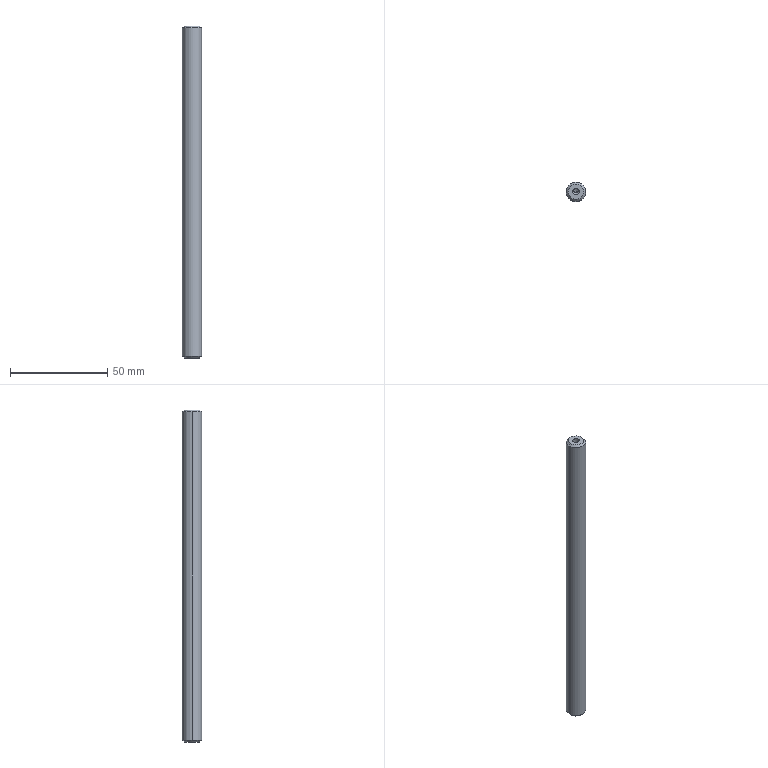Part | STEP file | PN_0005 Mount electronic clip support shaft | 1 solid | 16 faces | box 10 x 10 x 171 mm | volume 13199 mm3 | cone 8 | cylinder 6 | plane 2 | commonest cylinder face diameters 3.3 x4 10 x2
STEP:
#1=CARTESIAN_POINT('',(0.,0.,0.));
#2=DIRECTION('',(0.,0.,1.));
#3=DIRECTION('',(1.,0.,0.));
#4=AXIS2_PLACEMENT_3D('',#1,#2,#3);
#5=CARTESIAN_POINT('',(-1.65,0.,11.5));
#6=VERTEX_POINT('',#5);
#7=CARTESIAN_POINT('',(-1.65,0.,0.));
#8=VERTEX_POINT('',#7);
#9=CARTESIAN_POINT('',(-1.65,0.,0.));
#10=DIRECTION('',(0.,0.,-1.));
#11=VECTOR('',#10,1.);
#12=LINE('',#9,#11);
#13=CARTESIAN_POINT('',(0.,0.,0.));
#14=DIRECTION('',(0.,0.,-1.));
#15=DIRECTION('',(-1.,0.,0.));
#16=AXIS2_PLACEMENT_3D('',#13,#14,#15);
#17=CYLINDRICAL_SURFACE('',#16,1.65);
#18=CARTESIAN_POINT('',(6.283,0.));
#19=DIRECTION('',(0.,1.));
#20=VECTOR('',#19,1.);
#21=LINE('',#18,#20);
#22=(GEOMETRIC_REPRESENTATION_CONTEXT(2)PARAMETRIC_REPRESENTATION_CONTEXT()REPRESENTATION_CONTEXT('',''));
#23=DEFINITIONAL_REPRESENTATION('',(#21),#22);
#24=PCURVE('',#17,#23);
#25=CARTESIAN_POINT('',(0.,0.,0.));
#26=DIRECTION('',(0.,0.,-1.));
#27=DIRECTION('',(-1.,0.,0.));
#28=AXIS2_PLACEMENT_3D('',#25,#26,#27);
#29=CYLINDRICAL_SURFACE('',#28,1.65);
#30=CARTESIAN_POINT('',(0.,0.));
#31=DIRECTION('',(0.,1.));
#32=VECTOR('',#31,1.);
#33=LINE('',#30,#32);
#34=(GEOMETRIC_REPRESENTATION_CONTEXT(2)PARAMETRIC_REPRESENTATION_CONTEXT()REPRESENTATION_CONTEXT('',''));
#35=DEFINITIONAL_REPRESENTATION('',(#33),#34);
#36=PCURVE('',#29,#35);
#37=SURFACE_CURVE('',#12,(#24,#36),.PCURVE_S1.);
#38=EDGE_CURVE('',#6,#8,#37,.T.);
#39=ORIENTED_EDGE('',*,*,#38,.T.);
#40=CARTESIAN_POINT('',(1.65,0.,0.));
#41=VERTEX_POINT('',#40);
#42=CARTESIAN_POINT('',(0.,0.,0.));
#43=DIRECTION('',(0.,0.,-1.));
#44=DIRECTION('',(-1.,0.,0.));
#45=AXIS2_PLACEMENT_3D('',#42,#43,#44);
#46=CIRCLE('',#45,1.65);
#47=CARTESIAN_POINT('',(0.,0.));
#48=DIRECTION('',(1.,0.));
#49=VECTOR('',#48,1.);
#50=LINE('',#47,#49);
#51=(GEOMETRIC_REPRESENTATION_CONTEXT(2)PARAMETRIC_REPRESENTATION_CONTEXT()REPRESENTATION_CONTEXT('',''));
#52=DEFINITIONAL_REPRESENTATION('',(#50),#51);
#53=PCURVE('',#17,#52);
#54=CARTESIAN_POINT('',(0.,0.,0.));
#55=DIRECTION('',(0.,0.,1.));
#56=DIRECTION('',(1.,0.,0.));
#57=AXIS2_PLACEMENT_3D('',#54,#55,#56);
#58=PLANE('',#57);
#59=CARTESIAN_POINT('',(-1.65,0.));
#60=CARTESIAN_POINT('',(-1.65,2.858));
#61=CARTESIAN_POINT('',(0.825,1.429));
#62=CARTESIAN_POINT('',(3.3,0.));
#63=CARTESIAN_POINT('',(0.825,-1.429));
#64=CARTESIAN_POINT('',(-1.65,-2.858));
#65=CARTESIAN_POINT('',(-1.65,0.));
#66=(BOUNDED_CURVE()B_SPLINE_CURVE(2,(#59,#60,#61,#62,#63,#64,#65),.UNSPECIFIED.,.T.,.F.)B_SPLINE_CURVE_WITH_KNOTS((1,2,2,2,2,1),(-2.094,0.,2.094,4.189,6.283,8.378),.UNSPECIFIED.)CURVE()GEOMETRIC_REPRESENTATION_ITEM()RATIONAL_B_SPLINE_CURVE((1.,0.5,1.,0.5,1.,0.5,1.))REPRESENTATION_ITEM(''));
#67=(GEOMETRIC_REPRESENTATION_CONTEXT(2)PARAMETRIC_REPRESENTATION_CONTEXT()REPRESENTATION_CONTEXT('',''));
#68=DEFINITIONAL_REPRESENTATION('',(#66),#67);
#69=PCURVE('',#58,#68);
#70=SURFACE_CURVE('',#46,(#53,#69),.PCURVE_S1.);
#71=EDGE_CURVE('',#41,#8,#70,.T.);
#72=ORIENTED_EDGE('',*,*,#71,.F.);
#73=CARTESIAN_POINT('',(1.65,0.,11.5));
#74=VERTEX_POINT('',#73);
#75=CARTESIAN_POINT('',(1.65,0.,0.));
#76=DIRECTION('',(0.,0.,-1.));
#77=VECTOR('',#76,1.);
#78=LINE('',#75,#77);
#79=CARTESIAN_POINT('',(3.142,0.));
#80=DIRECTION('',(0.,1.));
#81=VECTOR('',#80,1.);
#82=LINE('',#79,#81);
#83=(GEOMETRIC_REPRESENTATION_CONTEXT(2)PARAMETRIC_REPRESENTATION_CONTEXT()REPRESENTATION_CONTEXT('',''));
#84=DEFINITIONAL_REPRESENTATION('',(#82),#83);
#85=PCURVE('',#17,#84);
#86=CARTESIAN_POINT('',(3.142,0.));
#87=DIRECTION('',(0.,1.));
#88=VECTOR('',#87,1.);
#89=LINE('',#86,#88);
#90=(GEOMETRIC_REPRESENTATION_CONTEXT(2)PARAMETRIC_REPRESENTATION_CONTEXT()REPRESENTATION_CONTEXT('',''));
#91=DEFINITIONAL_REPRESENTATION('',(#89),#90);
#92=PCURVE('',#29,#91);
#93=SURFACE_CURVE('',#78,(#85,#92),.PCURVE_S1.);
#94=EDGE_CURVE('',#74,#41,#93,.T.);
#95=ORIENTED_EDGE('',*,*,#94,.F.);
#96=CARTESIAN_POINT('',(0.,0.,11.5));
#97=DIRECTION('',(0.,0.,-1.));
#98=DIRECTION('',(-1.,0.,0.));
#99=AXIS2_PLACEMENT_3D('',#96,#97,#98);
#100=CIRCLE('',#99,1.65);
#101=CARTESIAN_POINT('',(0.,-11.5));
#102=DIRECTION('',(1.,0.));
#103=VECTOR('',#102,1.);
#104=LINE('',#101,#103);
#105=(GEOMETRIC_REPRESENTATION_CONTEXT(2)PARAMETRIC_REPRESENTATION_CONTEXT()REPRESENTATION_CONTEXT('',''));
#106=DEFINITIONAL_REPRESENTATION('',(#104),#105);
#107=PCURVE('',#17,#106);
#108=CARTESIAN_POINT('',(0.,0.,11.5));
#109=DIRECTION('',(0.,0.,-1.));
#110=DIRECTION('',(-1.,0.,0.));
#111=AXIS2_PLACEMENT_3D('',#108,#109,#110);
#112=CONICAL_SURFACE('',#111,1.65,1.03);
#113=CARTESIAN_POINT('',(0.,0.));
#114=DIRECTION('',(1.,0.));
#115=VECTOR('',#114,1.);
#116=LINE('',#113,#115);
#117=(GEOMETRIC_REPRESENTATION_CONTEXT(2)PARAMETRIC_REPRESENTATION_CONTEXT()REPRESENTATION_CONTEXT('',''));
#118=DEFINITIONAL_REPRESENTATION('',(#116),#117);
#119=PCURVE('',#112,#118);
#120=SURFACE_CURVE('',#100,(#107,#119),.PCURVE_S1.);
#121=EDGE_CURVE('',#74,#6,#120,.T.);
#122=ORIENTED_EDGE('',*,*,#121,.T.);
#123=EDGE_LOOP('',(#39,#72,#95,#122));
#124=FACE_BOUND('',#123,.F.);
#125=ADVANCED_FACE('',(#124),#17,.F.);
#126=ORIENTED_EDGE('',*,*,#121,.F.);
#127=CARTESIAN_POINT('',(0.,0.,12.491));
#128=VERTEX_POINT('',#127);
#129=CARTESIAN_POINT('',(1.65,0.,11.5));
#130=DIRECTION('',(0.8572,0.,-0.515));
#131=VECTOR('',#130,1.);
#132=LINE('',#129,#131);
#133=CARTESIAN_POINT('',(3.142,0.));
#134=DIRECTION('',(0.,1.));
#135=VECTOR('',#134,1.);
#136=LINE('',#133,#135);
#137=(GEOMETRIC_REPRESENTATION_CONTEXT(2)PARAMETRIC_REPRESENTATION_CONTEXT()REPRESENTATION_CONTEXT('',''));
#138=DEFINITIONAL_REPRESENTATION('',(#136),#137);
#139=PCURVE('',#112,#138);
#140=CARTESIAN_POINT('',(0.,0.,11.5));
#141=DIRECTION('',(0.,0.,-1.));
#142=DIRECTION('',(-1.,0.,0.));
#143=AXIS2_PLACEMENT_3D('',#140,#141,#142);
#144=CONICAL_SURFACE('',#143,1.65,1.03);
#145=CARTESIAN_POINT('',(3.142,0.));
#146=DIRECTION('',(0.,1.));
#147=VECTOR('',#146,1.);
#148=LINE('',#145,#147);
#149=(GEOMETRIC_REPRESENTATION_CONTEXT(2)PARAMETRIC_REPRESENTATION_CONTEXT()REPRESENTATION_CONTEXT('',''));
#150=DEFINITIONAL_REPRESENTATION('',(#148),#149);
#151=PCURVE('',#144,#150);
#152=SURFACE_CURVE('',#132,(#139,#151),.PCURVE_S1.);
#153=EDGE_CURVE('',#128,#74,#152,.T.);
#154=ORIENTED_EDGE('',*,*,#153,.F.);
#155=CARTESIAN_POINT('',(-1.65,0.,11.5));
#156=DIRECTION('',(-0.8572,0.,-0.515));
#157=VECTOR('',#156,1.);
#158=LINE('',#155,#157);
#159=CARTESIAN_POINT('',(6.283,0.));
#160=DIRECTION('',(0.,1.));
#161=VECTOR('',#160,1.);
#162=LINE('',#159,#161);
#163=(GEOMETRIC_REPRESENTATION_CONTEXT(2)PARAMETRIC_REPRESENTATION_CONTEXT()REPRESENTATION_CONTEXT('',''));
#164=DEFINITIONAL_REPRESENTATION('',(#162),#163);
#165=PCURVE('',#112,#164);
#166=CARTESIAN_POINT('',(0.,0.));
#167=DIRECTION('',(0.,1.));
#168=VECTOR('',#167,1.);
#169=LINE('',#166,#168);
#170=(GEOMETRIC_REPRESENTATION_CONTEXT(2)PARAMETRIC_REPRESENTATION_CONTEXT()REPRESENTATION_CONTEXT('',''));
#171=DEFINITIONAL_REPRESENTATION('',(#169),#170);
#172=PCURVE('',#144,#171);
#173=SURFACE_CURVE('',#158,(#165,#172),.PCURVE_S1.);
#174=EDGE_CURVE('',#128,#6,#173,.T.);
#175=ORIENTED_EDGE('',*,*,#174,.T.);
#176=EDGE_LOOP('',(#126,#154,#175));
#177=FACE_BOUND('',#176,.F.);
#178=ADVANCED_FACE('',(#177),#112,.F.);
#179=CARTESIAN_POINT('',(1.65,0.,159.5));
#180=VERTEX_POINT('',#179);
#181=CARTESIAN_POINT('',(1.65,0.,171.));
#182=VERTEX_POINT('',#181);
#183=CARTESIAN_POINT('',(1.65,0.,171.));
#184=DIRECTION('',(0.,0.,1.));
#185=VECTOR('',#184,1.);
#186=LINE('',#183,#185);
#187=CARTESIAN_POINT('',(0.,0.,171.));
#188=DIRECTION('',(0.,0.,1.));
#189=DIRECTION('',(1.,0.,0.));
#190=AXIS2_PLACEMENT_3D('',#187,#188,#189);
#191=CYLINDRICAL_SURFACE('',#190,1.65);
#192=CARTESIAN_POINT('',(6.283,0.));
#193=DIRECTION('',(0.,1.));
#194=VECTOR('',#193,1.);
#195=LINE('',#192,#194);
#196=(GEOMETRIC_REPRESENTATION_CONTEXT(2)PARAMETRIC_REPRESENTATION_CONTEXT()REPRESENTATION_CONTEXT('',''));
#197=DEFINITIONAL_REPRESENTATION('',(#195),#196);
#198=PCURVE('',#191,#197);
#199=CARTESIAN_POINT('',(0.,0.,171.));
#200=DIRECTION('',(0.,0.,1.));
#201=DIRECTION('',(1.,0.,0.));
#202=AXIS2_PLACEMENT_3D('',#199,#200,#201);
#203=CYLINDRICAL_SURFACE('',#202,1.65);
#204=CARTESIAN_POINT('',(0.,0.));
#205=DIRECTION('',(0.,1.));
#206=VECTOR('',#205,1.);
#207=LINE('',#204,#206);
#208=(GEOMETRIC_REPRESENTATION_CONTEXT(2)PARAMETRIC_REPRESENTATION_CONTEXT()REPRESENTATION_CONTEXT('',''));
#209=DEFINITIONAL_REPRESENTATION('',(#207),#208);
#210=PCURVE('',#203,#209);
#211=SURFACE_CURVE('',#186,(#198,#210),.PCURVE_S1.);
#212=EDGE_CURVE('',#180,#182,#211,.T.);
#213=ORIENTED_EDGE('',*,*,#212,.T.);
#214=CARTESIAN_POINT('',(-1.65,0.,171.));
#215=VERTEX_POINT('',#214);
#216=CARTESIAN_POINT('',(0.,0.,171.));
#217=DIRECTION('',(0.,0.,1.));
#218=DIRECTION('',(1.,0.,0.));
#219=AXIS2_PLACEMENT_3D('',#216,#217,#218);
#220=CIRCLE('',#219,1.65);
#221=CARTESIAN_POINT('',(0.,0.));
#222=DIRECTION('',(1.,0.));
#223=VECTOR('',#222,1.);
#224=LINE('',#221,#223);
#225=(GEOMETRIC_REPRESENTATION_CONTEXT(2)PARAMETRIC_REPRESENTATION_CONTEXT()REPRESENTATION_CONTEXT('',''));
#226=DEFINITIONAL_REPRESENTATION('',(#224),#225);
#227=PCURVE('',#191,#226);
#228=CARTESIAN_POINT('',(0.,0.,171.));
#229=DIRECTION('',(0.,0.,1.));
#230=DIRECTION('',(1.,0.,0.));
#231=AXIS2_PLACEMENT_3D('',#228,#229,#230);
#232=PLANE('',#231);
#233=CARTESIAN_POINT('',(0.,0.));
#234=DIRECTION('',(1.,0.));
#235=AXIS2_PLACEMENT_2D('',#233,#234);
#236=CIRCLE('',#235,1.65);
#237=(GEOMETRIC_REPRESENTATION_CONTEXT(2)PARAMETRIC_REPRESENTATION_CONTEXT()REPRESENTATION_CONTEXT('',''));
#238=DEFINITIONAL_REPRESENTATION('',(#236),#237);
#239=PCURVE('',#232,#238);
#240=SURFACE_CURVE('',#220,(#227,#239),.PCURVE_S1.);
#241=EDGE_CURVE('',#215,#182,#240,.T.);
#242=ORIENTED_EDGE('',*,*,#241,.F.);
#243=CARTESIAN_POINT('',(-1.65,0.,159.5));
#244=VERTEX_POINT('',#243);
#245=CARTESIAN_POINT('',(-1.65,0.,171.));
#246=DIRECTION('',(0.,0.,1.));
#247=VECTOR('',#246,1.);
#248=LINE('',#245,#247);
#249=CARTESIAN_POINT('',(3.142,0.));
#250=DIRECTION('',(0.,1.));
#251=VECTOR('',#250,1.);
#252=LINE('',#249,#251);
#253=(GEOMETRIC_REPRESENTATION_CONTEXT(2)PARAMETRIC_REPRESENTATION_CONTEXT()REPRESENTATION_CONTEXT('',''));
#254=DEFINITIONAL_REPRESENTATION('',(#252),#253);
#255=PCURVE('',#191,#254);
#256=CARTESIAN_POINT('',(3.142,0.));
#257=DIRECTION('',(0.,1.));
#258=VECTOR('',#257,1.);
#259=LINE('',#256,#258);
#260=(GEOMETRIC_REPRESENTATION_CONTEXT(2)PARAMETRIC_REPRESENTATION_CONTEXT()REPRESENTATION_CONTEXT('',''));
#261=DEFINITIONAL_REPRESENTATION('',(#259),#260);
#262=PCURVE('',#203,#261);
#263=SURFACE_CURVE('',#248,(#255,#262),.PCURVE_S1.);
#264=EDGE_CURVE('',#244,#215,#263,.T.);
#265=ORIENTED_EDGE('',*,*,#264,.F.);
#266=CARTESIAN_POINT('',(0.,0.,159.5));
#267=DIRECTION('',(0.,0.,1.));
#268=DIRECTION('',(1.,0.,0.));
#269=AXIS2_PLACEMENT_3D('',#266,#267,#268);
#270=CIRCLE('',#269,1.65);
#271=CARTESIAN_POINT('',(0.,-11.5));
#272=DIRECTION('',(1.,0.));
#273=VECTOR('',#272,1.);
#274=LINE('',#271,#273);
#275=(GEOMETRIC_REPRESENTATION_CONTEXT(2)PARAMETRIC_REPRESENTATION_CONTEXT()REPRESENTATION_CONTEXT('',''));
#276=DEFINITIONAL_REPRESENTATION('',(#274),#275);
#277=PCURVE('',#191,#276);
#278=CARTESIAN_POINT('',(0.,0.,159.5));
#279=DIRECTION('',(0.,0.,1.));
#280=DIRECTION('',(1.,0.,0.));
#281=AXIS2_PLACEMENT_3D('',#278,#279,#280);
#282=CONICAL_SURFACE('',#281,1.65,1.03);
#283=CARTESIAN_POINT('',(0.,0.));
#284=DIRECTION('',(1.,0.));
#285=VECTOR('',#284,1.);
#286=LINE('',#283,#285);
#287=(GEOMETRIC_REPRESENTATION_CONTEXT(2)PARAMETRIC_REPRESENTATION_CONTEXT()REPRESENTATION_CONTEXT('',''));
#288=DEFINITIONAL_REPRESENTATION('',(#286),#287);
#289=PCURVE('',#282,#288);
#290=SURFACE_CURVE('',#270,(#277,#289),.PCURVE_S1.);
#291=EDGE_CURVE('',#244,#180,#290,.T.);
#292=ORIENTED_EDGE('',*,*,#291,.T.);
#293=EDGE_LOOP('',(#213,#242,#265,#292));
#294=FACE_BOUND('',#293,.F.);
#295=ADVANCED_FACE('',(#294),#191,.F.);
#296=ORIENTED_EDGE('',*,*,#291,.F.);
#297=CARTESIAN_POINT('',(0.,0.,158.509));
#298=VERTEX_POINT('',#297);
#299=CARTESIAN_POINT('',(-1.65,0.,159.5));
#300=DIRECTION('',(-0.8572,0.,0.515));
#301=VECTOR('',#300,1.);
#302=LINE('',#299,#301);
#303=CARTESIAN_POINT('',(3.142,0.));
#304=DIRECTION('',(0.,1.));
#305=VECTOR('',#304,1.);
#306=LINE('',#303,#305);
#307=(GEOMETRIC_REPRESENTATION_CONTEXT(2)PARAMETRIC_REPRESENTATION_CONTEXT()REPRESENTATION_CONTEXT('',''));
#308=DEFINITIONAL_REPRESENTATION('',(#306),#307);
#309=PCURVE('',#282,#308);
#310=CARTESIAN_POINT('',(0.,0.,159.5));
#311=DIRECTION('',(0.,0.,1.));
#312=DIRECTION('',(1.,0.,0.));
#313=AXIS2_PLACEMENT_3D('',#310,#311,#312);
#314=CONICAL_SURFACE('',#313,1.65,1.03);
#315=CARTESIAN_POINT('',(3.142,0.));
#316=DIRECTION('',(0.,1.));
#317=VECTOR('',#316,1.);
#318=LINE('',#315,#317);
#319=(GEOMETRIC_REPRESENTATION_CONTEXT(2)PARAMETRIC_REPRESENTATION_CONTEXT()REPRESENTATION_CONTEXT('',''));
#320=DEFINITIONAL_REPRESENTATION('',(#318),#319);
#321=PCURVE('',#314,#320);
#322=SURFACE_CURVE('',#302,(#309,#321),.PCURVE_S1.);
#323=EDGE_CURVE('',#298,#244,#322,.T.);
#324=ORIENTED_EDGE('',*,*,#323,.F.);
#325=CARTESIAN_POINT('',(1.65,0.,159.5));
#326=DIRECTION('',(0.8572,0.,0.515));
#327=VECTOR('',#326,1.);
#328=LINE('',#325,#327);
#329=CARTESIAN_POINT('',(6.283,0.));
#330=DIRECTION('',(0.,1.));
#331=VECTOR('',#330,1.);
#332=LINE('',#329,#331);
#333=(GEOMETRIC_REPRESENTATION_CONTEXT(2)PARAMETRIC_REPRESENTATION_CONTEXT()REPRESENTATION_CONTEXT('',''));
#334=DEFINITIONAL_REPRESENTATION('',(#332),#333);
#335=PCURVE('',#282,#334);
#336=CARTESIAN_POINT('',(0.,0.));
#337=DIRECTION('',(0.,1.));
#338=VECTOR('',#337,1.);
#339=LINE('',#336,#338);
#340=(GEOMETRIC_REPRESENTATION_CONTEXT(2)PARAMETRIC_REPRESENTATION_CONTEXT()REPRESENTATION_CONTEXT('',''));
#341=DEFINITIONAL_REPRESENTATION('',(#339),#340);
#342=PCURVE('',#314,#341);
#343=SURFACE_CURVE('',#328,(#335,#342),.PCURVE_S1.);
#344=EDGE_CURVE('',#298,#180,#343,.T.);
#345=ORIENTED_EDGE('',*,*,#344,.T.);
#346=EDGE_LOOP('',(#296,#324,#345));
#347=FACE_BOUND('',#346,.F.);
#348=ADVANCED_FACE('',(#347),#282,.F.);
#349=CARTESIAN_POINT('',(4.,0.,171.));
#350=VERTEX_POINT('',#349);
#351=CARTESIAN_POINT('',(-4.,0.,171.));
#352=VERTEX_POINT('',#351);
#353=CARTESIAN_POINT('',(0.,0.,171.));
#354=DIRECTION('',(0.,0.,1.));
#355=DIRECTION('',(1.,0.,0.));
#356=AXIS2_PLACEMENT_3D('',#353,#354,#355);
#357=CIRCLE('',#356,4.);
#358=CARTESIAN_POINT('',(0.,0.,171.));
#359=DIRECTION('',(0.,0.,-1.));
#360=DIRECTION('',(-1.,0.,0.));
#361=AXIS2_PLACEMENT_3D('',#358,#359,#360);
#362=CONICAL_SURFACE('',#361,4.,0.7854);
#363=CARTESIAN_POINT('',(3.142,0.));
#364=DIRECTION('',(-1.,0.));
#365=VECTOR('',#364,1.);
#366=LINE('',#363,#365);
#367=(GEOMETRIC_REPRESENTATION_CONTEXT(2)PARAMETRIC_REPRESENTATION_CONTEXT()REPRESENTATION_CONTEXT('',''));
#368=DEFINITIONAL_REPRESENTATION('',(#366),#367);
#369=PCURVE('',#362,#368);
#370=CARTESIAN_POINT('',(0.,0.));
#371=DIRECTION('',(1.,0.));
#372=AXIS2_PLACEMENT_2D('',#370,#371);
#373=CIRCLE('',#372,4.);
#374=(GEOMETRIC_REPRESENTATION_CONTEXT(2)PARAMETRIC_REPRESENTATION_CONTEXT()REPRESENTATION_CONTEXT('',''));
#375=DEFINITIONAL_REPRESENTATION('',(#373),#374);
#376=PCURVE('',#232,#375);
#377=SURFACE_CURVE('',#357,(#369,#376),.PCURVE_S1.);
#378=EDGE_CURVE('',#350,#352,#377,.T.);
#379=ORIENTED_EDGE('',*,*,#378,.F.);
#380=CARTESIAN_POINT('',(5.,0.,170.));
#381=VERTEX_POINT('',#380);
#382=CARTESIAN_POINT('',(4.,0.,171.));
#383=DIRECTION('',(0.7071,0.,-0.7071));
#384=VECTOR('',#383,1.);
#385=LINE('',#382,#384);
#386=CARTESIAN_POINT('',(3.142,0.));
#387=DIRECTION('',(0.,1.));
#388=VECTOR('',#387,1.);
#389=LINE('',#386,#388);
#390=(GEOMETRIC_REPRESENTATION_CONTEXT(2)PARAMETRIC_REPRESENTATION_CONTEXT()REPRESENTATION_CONTEXT('',''));
#391=DEFINITIONAL_REPRESENTATION('',(#389),#390);
#392=PCURVE('',#362,#391);
#393=CARTESIAN_POINT('',(0.,0.,171.));
#394=DIRECTION('',(0.,0.,-1.));
#395=DIRECTION('',(-1.,0.,0.));
#396=AXIS2_PLACEMENT_3D('',#393,#394,#395);
#397=CONICAL_SURFACE('',#396,4.,0.7854);
#398=CARTESIAN_POINT('',(3.142,0.));
#399=DIRECTION('',(0.,1.));
#400=VECTOR('',#399,1.);
#401=LINE('',#398,#400);
#402=(GEOMETRIC_REPRESENTATION_CONTEXT(2)PARAMETRIC_REPRESENTATION_CONTEXT()REPRESENTATION_CONTEXT('',''));
#403=DEFINITIONAL_REPRESENTATION('',(#401),#402);
#404=PCURVE('',#397,#403);
#405=SURFACE_CURVE('',#385,(#392,#404),.PCURVE_S1.);
#406=EDGE_CURVE('',#350,#381,#405,.T.);
#407=ORIENTED_EDGE('',*,*,#406,.T.);
#408=CARTESIAN_POINT('',(-5.,0.,170.));
#409=VERTEX_POINT('',#408);
#410=CARTESIAN_POINT('',(0.,0.,170.));
#411=DIRECTION('',(0.,0.,-1.));
#412=DIRECTION('',(1.,0.,0.));
#413=AXIS2_PLACEMENT_3D('',#410,#411,#412);
#414=CIRCLE('',#413,5.);
#415=CARTESIAN_POINT('',(-3.142,1.));
#416=DIRECTION('',(1.,0.));
#417=VECTOR('',#416,1.);
#418=LINE('',#415,#417);
#419=(GEOMETRIC_REPRESENTATION_CONTEXT(2)PARAMETRIC_REPRESENTATION_CONTEXT()REPRESENTATION_CONTEXT('',''));
#420=DEFINITIONAL_REPRESENTATION('',(#418),#419);
#421=PCURVE('',#362,#420);
#422=CARTESIAN_POINT('',(0.,0.,171.));
#423=DIRECTION('',(0.,0.,-1.));
#424=DIRECTION('',(-1.,0.,0.));
#425=AXIS2_PLACEMENT_3D('',#422,#423,#424);
#426=CYLINDRICAL_SURFACE('',#425,5.);
#427=CARTESIAN_POINT('',(-3.142,1.));
#428=DIRECTION('',(1.,0.));
#429=VECTOR('',#428,1.);
#430=LINE('',#427,#429);
#431=(GEOMETRIC_REPRESENTATION_CONTEXT(2)PARAMETRIC_REPRESENTATION_CONTEXT()REPRESENTATION_CONTEXT('',''));
#432=DEFINITIONAL_REPRESENTATION('',(#430),#431);
#433=PCURVE('',#426,#432);
#434=SURFACE_CURVE('',#414,(#421,#433),.PCURVE_S1.);
#435=EDGE_CURVE('',#409,#381,#434,.T.);
#436=ORIENTED_EDGE('',*,*,#435,.F.);
#437=CARTESIAN_POINT('',(-4.,0.,171.));
#438=DIRECTION('',(-0.7071,0.,-0.7071));
#439=VECTOR('',#438,1.);
#440=LINE('',#437,#439);
#441=CARTESIAN_POINT('',(0.,0.));
#442=DIRECTION('',(0.,1.));
#443=VECTOR('',#442,1.);
#444=LINE('',#441,#443);
#445=(GEOMETRIC_REPRESENTATION_CONTEXT(2)PARAMETRIC_REPRESENTATION_CONTEXT()REPRESENTATION_CONTEXT('',''));
#446=DEFINITIONAL_REPRESENTATION('',(#444),#445);
#447=PCURVE('',#362,#446);
#448=CARTESIAN_POINT('',(6.283,0.));
#449=DIRECTION('',(0.,1.));
#450=VECTOR('',#449,1.);
#451=LINE('',#448,#450);
#452=(GEOMETRIC_REPRESENTATION_CONTEXT(2)PARAMETRIC_REPRESENTATION_CONTEXT()REPRESENTATION_CONTEXT('',''));
#453=DEFINITIONAL_REPRESENTATION('',(#451),#452);
#454=PCURVE('',#397,#453);
#455=SURFACE_CURVE('',#440,(#447,#454),.PCURVE_S1.);
#456=EDGE_CURVE('',#352,#409,#455,.T.);
#457=ORIENTED_EDGE('',*,*,#456,.F.);
#458=EDGE_LOOP('',(#379,#407,#436,#457));
#459=FACE_BOUND('',#458,.T.);
#460=ADVANCED_FACE('',(#459),#362,.T.);
#461=CARTESIAN_POINT('',(-4.,0.,0.));
#462=VERTEX_POINT('',#461);
#463=CARTESIAN_POINT('',(4.,0.,0.));
#464=VERTEX_POINT('',#463);
#465=CARTESIAN_POINT('',(0.,0.,0.));
#466=DIRECTION('',(0.,0.,-1.));
#467=DIRECTION('',(1.,0.,0.));
#468=AXIS2_PLACEMENT_3D('',#465,#466,#467);
#469=CIRCLE('',#468,4.);
#470=CARTESIAN_POINT('',(0.,0.,1.));
#471=DIRECTION('',(0.,0.,1.));
#472=DIRECTION('',(1.,0.,0.));
#473=AXIS2_PLACEMENT_3D('',#470,#471,#472);
#474=CONICAL_SURFACE('',#473,5.,0.7854);
#475=CARTESIAN_POINT('',(6.283,-1.));
#476=DIRECTION('',(-1.,0.));
#477=VECTOR('',#476,1.);
#478=LINE('',#475,#477);
#479=(GEOMETRIC_REPRESENTATION_CONTEXT(2)PARAMETRIC_REPRESENTATION_CONTEXT()REPRESENTATION_CONTEXT('',''));
#480=DEFINITIONAL_REPRESENTATION('',(#478),#479);
#481=PCURVE('',#474,#480);
#482=CARTESIAN_POINT('',(4.,0.));
#483=CARTESIAN_POINT('',(4.,-6.928));
#484=CARTESIAN_POINT('',(-2.,-3.464));
#485=CARTESIAN_POINT('',(-8.,0.));
#486=CARTESIAN_POINT('',(-2.,3.464));
#487=CARTESIAN_POINT('',(4.,6.928));
#488=CARTESIAN_POINT('',(4.,0.));
#489=(BOUNDED_CURVE()B_SPLINE_CURVE(2,(#482,#483,#484,#485,#486,#487,#488),.UNSPECIFIED.,.T.,.F.)B_SPLINE_CURVE_WITH_KNOTS((1,2,2,2,2,1),(-2.094,0.,2.094,4.189,6.283,8.378),.UNSPECIFIED.)CURVE()GEOMETRIC_REPRESENTATION_ITEM()RATIONAL_B_SPLINE_CURVE((1.,0.5,1.,0.5,1.,0.5,1.))REPRESENTATION_ITEM(''));
#490=(GEOMETRIC_REPRESENTATION_CONTEXT(2)PARAMETRIC_REPRESENTATION_CONTEXT()REPRESENTATION_CONTEXT('',''));
#491=DEFINITIONAL_REPRESENTATION('',(#489),#490);
#492=PCURVE('',#58,#491);
#493=SURFACE_CURVE('',#469,(#481,#492),.PCURVE_S1.);
#494=EDGE_CURVE('',#462,#464,#493,.T.);
#495=ORIENTED_EDGE('',*,*,#494,.F.);
#496=CARTESIAN_POINT('',(-5.,0.,1.));
#497=VERTEX_POINT('',#496);
#498=CARTESIAN_POINT('',(-5.,0.,1.));
#499=DIRECTION('',(-0.7071,0.,0.7071));
#500=VECTOR('',#499,1.);
#501=LINE('',#498,#500);
#502=CARTESIAN_POINT('',(3.142,0.));
#503=DIRECTION('',(0.,1.));
#504=VECTOR('',#503,1.);
#505=LINE('',#502,#504);
#506=(GEOMETRIC_REPRESENTATION_CONTEXT(2)PARAMETRIC_REPRESENTATION_CONTEXT()REPRESENTATION_CONTEXT('',''));
#507=DEFINITIONAL_REPRESENTATION('',(#505),#506);
#508=PCURVE('',#474,#507);
#509=CARTESIAN_POINT('',(0.,0.,1.));
#510=DIRECTION('',(0.,0.,1.));
#511=DIRECTION('',(1.,0.,0.));
#512=AXIS2_PLACEMENT_3D('',#509,#510,#511);
#513=CONICAL_SURFACE('',#512,5.,0.7854);
#514=CARTESIAN_POINT('',(3.142,0.));
#515=DIRECTION('',(0.,1.));
#516=VECTOR('',#515,1.);
#517=LINE('',#514,#516);
#518=(GEOMETRIC_REPRESENTATION_CONTEXT(2)PARAMETRIC_REPRESENTATION_CONTEXT()REPRESENTATION_CONTEXT('',''));
#519=DEFINITIONAL_REPRESENTATION('',(#517),#518);
#520=PCURVE('',#513,#519);
#521=SURFACE_CURVE('',#501,(#508,#520),.PCURVE_S1.);
#522=EDGE_CURVE('',#462,#497,#521,.T.);
#523=ORIENTED_EDGE('',*,*,#522,.T.);
#524=CARTESIAN_POINT('',(5.,0.,1.));
#525=VERTEX_POINT('',#524);
#526=CARTESIAN_POINT('',(0.,0.,1.));
#527=DIRECTION('',(0.,0.,1.));
#528=DIRECTION('',(1.,0.,0.));
#529=AXIS2_PLACEMENT_3D('',#526,#527,#528);
#530=CIRCLE('',#529,5.);
#531=CARTESIAN_POINT('',(0.,0.));
#532=DIRECTION('',(1.,0.));
#533=VECTOR('',#532,1.);
#534=LINE('',#531,#533);
#535=(GEOMETRIC_REPRESENTATION_CONTEXT(2)PARAMETRIC_REPRESENTATION_CONTEXT()REPRESENTATION_CONTEXT('',''));
#536=DEFINITIONAL_REPRESENTATION('',(#534),#535);
#537=PCURVE('',#474,#536);
#538=CARTESIAN_POINT('',(3.142,170.));
#539=DIRECTION('',(-1.,0.));
#540=VECTOR('',#539,1.);
#541=LINE('',#538,#540);
#542=(GEOMETRIC_REPRESENTATION_CONTEXT(2)PARAMETRIC_REPRESENTATION_CONTEXT()REPRESENTATION_CONTEXT('',''));
#543=DEFINITIONAL_REPRESENTATION('',(#541),#542);
#544=PCURVE('',#426,#543);
#545=SURFACE_CURVE('',#530,(#537,#544),.PCURVE_S1.);
#546=EDGE_CURVE('',#525,#497,#545,.T.);
#547=ORIENTED_EDGE('',*,*,#546,.F.);
#548=CARTESIAN_POINT('',(5.,0.,1.));
#549=DIRECTION('',(0.7071,0.,0.7071));
#550=VECTOR('',#549,1.);
#551=LINE('',#548,#550);
#552=CARTESIAN_POINT('',(0.,0.));
#553=DIRECTION('',(0.,1.));
#554=VECTOR('',#553,1.);
#555=LINE('',#552,#554);
#556=(GEOMETRIC_REPRESENTATION_CONTEXT(2)PARAMETRIC_REPRESENTATION_CONTEXT()REPRESENTATION_CONTEXT('',''));
#557=DEFINITIONAL_REPRESENTATION('',(#555),#556);
#558=PCURVE('',#474,#557);
#559=CARTESIAN_POINT('',(6.283,0.));
#560=DIRECTION('',(0.,1.));
#561=VECTOR('',#560,1.);
#562=LINE('',#559,#561);
#563=(GEOMETRIC_REPRESENTATION_CONTEXT(2)PARAMETRIC_REPRESENTATION_CONTEXT()REPRESENTATION_CONTEXT('',''));
#564=DEFINITIONAL_REPRESENTATION('',(#562),#563);
#565=PCURVE('',#513,#564);
#566=SURFACE_CURVE('',#551,(#558,#565),.PCURVE_S1.);
#567=EDGE_CURVE('',#464,#525,#566,.T.);
#568=ORIENTED_EDGE('',*,*,#567,.F.);
#569=EDGE_LOOP('',(#495,#523,#547,#568));
#570=FACE_BOUND('',#569,.T.);
#571=ADVANCED_FACE('',(#570),#474,.T.);
#572=ORIENTED_EDGE('',*,*,#435,.T.);
#573=CARTESIAN_POINT('',(5.,0.,171.));
#574=DIRECTION('',(0.,0.,-1.));
#575=VECTOR('',#574,1.);
#576=LINE('',#573,#575);
#577=CARTESIAN_POINT('',(3.142,0.));
#578=DIRECTION('',(0.,1.));
#579=VECTOR('',#578,1.);
#580=LINE('',#577,#579);
#581=(GEOMETRIC_REPRESENTATION_CONTEXT(2)PARAMETRIC_REPRESENTATION_CONTEXT()REPRESENTATION_CONTEXT('',''));
#582=DEFINITIONAL_REPRESENTATION('',(#580),#581);
#583=PCURVE('',#426,#582);
#584=CARTESIAN_POINT('',(0.,0.,171.));
#585=DIRECTION('',(0.,0.,-1.));
#586=DIRECTION('',(-1.,0.,0.));
#587=AXIS2_PLACEMENT_3D('',#584,#585,#586);
#588=CYLINDRICAL_SURFACE('',#587,5.);
#589=CARTESIAN_POINT('',(3.142,0.));
#590=DIRECTION('',(0.,1.));
#591=VECTOR('',#590,1.);
#592=LINE('',#589,#591);
#593=(GEOMETRIC_REPRESENTATION_CONTEXT(2)PARAMETRIC_REPRESENTATION_CONTEXT()REPRESENTATION_CONTEXT('',''));
#594=DEFINITIONAL_REPRESENTATION('',(#592),#593);
#595=PCURVE('',#588,#594);
#596=SURFACE_CURVE('',#576,(#583,#595),.PCURVE_S1.);
#597=EDGE_CURVE('',#381,#525,#596,.T.);
#598=ORIENTED_EDGE('',*,*,#597,.T.);
#599=ORIENTED_EDGE('',*,*,#546,.T.);
#600=CARTESIAN_POINT('',(-5.,0.,171.));
#601=DIRECTION('',(0.,0.,-1.));
#602=VECTOR('',#601,1.);
#603=LINE('',#600,#602);
#604=CARTESIAN_POINT('',(0.,0.));
#605=DIRECTION('',(0.,1.));
#606=VECTOR('',#605,1.);
#607=LINE('',#604,#606);
#608=(GEOMETRIC_REPRESENTATION_CONTEXT(2)PARAMETRIC_REPRESENTATION_CONTEXT()REPRESENTATION_CONTEXT('',''));
#609=DEFINITIONAL_REPRESENTATION('',(#607),#608);
#610=PCURVE('',#426,#609);
#611=CARTESIAN_POINT('',(6.283,0.));
#612=DIRECTION('',(0.,1.));
#613=VECTOR('',#612,1.);
#614=LINE('',#611,#613);
#615=(GEOMETRIC_REPRESENTATION_CONTEXT(2)PARAMETRIC_REPRESENTATION_CONTEXT()REPRESENTATION_CONTEXT('',''));
#616=DEFINITIONAL_REPRESENTATION('',(#614),#615);
#617=PCURVE('',#588,#616);
#618=SURFACE_CURVE('',#603,(#610,#617),.PCURVE_S1.);
#619=EDGE_CURVE('',#409,#497,#618,.T.);
#620=ORIENTED_EDGE('',*,*,#619,.F.);
#621=EDGE_LOOP('',(#572,#598,#599,#620));
#622=FACE_BOUND('',#621,.T.);
#623=ADVANCED_FACE('',(#622),#426,.T.);
#624=ORIENTED_EDGE('',*,*,#597,.F.);
#625=CARTESIAN_POINT('',(0.,0.,170.));
#626=DIRECTION('',(0.,0.,-1.));
#627=DIRECTION('',(1.,0.,0.));
#628=AXIS2_PLACEMENT_3D('',#625,#626,#627);
#629=CIRCLE('',#628,5.);
#630=CARTESIAN_POINT('',(3.142,1.));
#631=DIRECTION('',(1.,0.));
#632=VECTOR('',#631,1.);
#633=LINE('',#630,#632);
#634=(GEOMETRIC_REPRESENTATION_CONTEXT(2)PARAMETRIC_REPRESENTATION_CONTEXT()REPRESENTATION_CONTEXT('',''));
#635=DEFINITIONAL_REPRESENTATION('',(#633),#634);
#636=PCURVE('',#588,#635);
#637=CARTESIAN_POINT('',(3.142,1.));
#638=DIRECTION('',(1.,0.));
#639=VECTOR('',#638,1.);
#640=LINE('',#637,#639);
#641=(GEOMETRIC_REPRESENTATION_CONTEXT(2)PARAMETRIC_REPRESENTATION_CONTEXT()REPRESENTATION_CONTEXT('',''));
#642=DEFINITIONAL_REPRESENTATION('',(#640),#641);
#643=PCURVE('',#397,#642);
#644=SURFACE_CURVE('',#629,(#636,#643),.PCURVE_S1.);
#645=EDGE_CURVE('',#381,#409,#644,.T.);
#646=ORIENTED_EDGE('',*,*,#645,.T.);
#647=ORIENTED_EDGE('',*,*,#619,.T.);
#648=CARTESIAN_POINT('',(0.,0.,1.));
#649=DIRECTION('',(0.,0.,1.));
#650=DIRECTION('',(1.,0.,0.));
#651=AXIS2_PLACEMENT_3D('',#648,#649,#650);
#652=CIRCLE('',#651,5.);
#653=CARTESIAN_POINT('',(9.425,170.));
#654=DIRECTION('',(-1.,0.));
#655=VECTOR('',#654,1.);
#656=LINE('',#653,#655);
#657=(GEOMETRIC_REPRESENTATION_CONTEXT(2)PARAMETRIC_REPRESENTATION_CONTEXT()REPRESENTATION_CONTEXT('',''));
#658=DEFINITIONAL_REPRESENTATION('',(#656),#657);
#659=PCURVE('',#588,#658);
#660=CARTESIAN_POINT('',(0.,0.));
#661=DIRECTION('',(1.,0.));
#662=VECTOR('',#661,1.);
#663=LINE('',#660,#662);
#664=(GEOMETRIC_REPRESENTATION_CONTEXT(2)PARAMETRIC_REPRESENTATION_CONTEXT()REPRESENTATION_CONTEXT('',''));
#665=DEFINITIONAL_REPRESENTATION('',(#663),#664);
#666=PCURVE('',#513,#665);
#667=SURFACE_CURVE('',#652,(#659,#666),.PCURVE_S1.);
#668=EDGE_CURVE('',#497,#525,#667,.T.);
#669=ORIENTED_EDGE('',*,*,#668,.T.);
#670=EDGE_LOOP('',(#624,#646,#647,#669));
#671=FACE_BOUND('',#670,.T.);
#672=ADVANCED_FACE('',(#671),#588,.T.);
#673=CARTESIAN_POINT('',(0.,0.,171.));
#674=DIRECTION('',(0.,0.,1.));
#675=DIRECTION('',(1.,0.,0.));
#676=AXIS2_PLACEMENT_3D('',#673,#674,#675);
#677=CIRCLE('',#676,1.65);
#678=CARTESIAN_POINT('',(0.,0.));
#679=DIRECTION('',(1.,0.));
#680=AXIS2_PLACEMENT_2D('',#678,#679);
#681=CIRCLE('',#680,1.65);
#682=(GEOMETRIC_REPRESENTATION_CONTEXT(2)PARAMETRIC_REPRESENTATION_CONTEXT()REPRESENTATION_CONTEXT('',''));
#683=DEFINITIONAL_REPRESENTATION('',(#681),#682);
#684=PCURVE('',#232,#683);
#685=CARTESIAN_POINT('',(0.,0.));
#686=DIRECTION('',(1.,0.));
#687=VECTOR('',#686,1.);
#688=LINE('',#685,#687);
#689=(GEOMETRIC_REPRESENTATION_CONTEXT(2)PARAMETRIC_REPRESENTATION_CONTEXT()REPRESENTATION_CONTEXT('',''));
#690=DEFINITIONAL_REPRESENTATION('',(#688),#689);
#691=PCURVE('',#203,#690);
#692=SURFACE_CURVE('',#677,(#684,#691),.PCURVE_S1.);
#693=EDGE_CURVE('',#182,#215,#692,.T.);
#694=ORIENTED_EDGE('',*,*,#693,.F.);
#695=ORIENTED_EDGE('',*,*,#241,.F.);
#696=EDGE_LOOP('',(#694,#695));
#697=FACE_BOUND('',#696,.T.);
#698=CARTESIAN_POINT('',(0.,0.,171.));
#699=DIRECTION('',(0.,0.,1.));
#700=DIRECTION('',(1.,0.,0.));
#701=AXIS2_PLACEMENT_3D('',#698,#699,#700);
#702=CIRCLE('',#701,4.);
#703=CARTESIAN_POINT('',(0.,0.));
#704=DIRECTION('',(1.,0.));
#705=AXIS2_PLACEMENT_2D('',#703,#704);
#706=CIRCLE('',#705,4.);
#707=(GEOMETRIC_REPRESENTATION_CONTEXT(2)PARAMETRIC_REPRESENTATION_CONTEXT()REPRESENTATION_CONTEXT('',''));
#708=DEFINITIONAL_REPRESENTATION('',(#706),#707);
#709=PCURVE('',#232,#708);
#710=CARTESIAN_POINT('',(9.425,0.));
#711=DIRECTION('',(-1.,0.));
#712=VECTOR('',#711,1.);
#713=LINE('',#710,#712);
#714=(GEOMETRIC_REPRESENTATION_CONTEXT(2)PARAMETRIC_REPRESENTATION_CONTEXT()REPRESENTATION_CONTEXT('',''));
#715=DEFINITIONAL_REPRESENTATION('',(#713),#714);
#716=PCURVE('',#397,#715);
#717=SURFACE_CURVE('',#702,(#709,#716),.PCURVE_S1.);
#718=EDGE_CURVE('',#352,#350,#717,.T.);
#719=ORIENTED_EDGE('',*,*,#718,.T.);
#720=ORIENTED_EDGE('',*,*,#378,.T.);
#721=EDGE_LOOP('',(#719,#720));
#722=FACE_BOUND('',#721,.T.);
#723=ADVANCED_FACE('',(#697,#722),#232,.T.);
#724=CARTESIAN_POINT('',(0.,0.,0.));
#725=DIRECTION('',(0.,0.,-1.));
#726=DIRECTION('',(-1.,0.,0.));
#727=AXIS2_PLACEMENT_3D('',#724,#725,#726);
#728=CIRCLE('',#727,1.65);
#729=CARTESIAN_POINT('',(-1.65,0.));
#730=CARTESIAN_POINT('',(-1.65,2.858));
#731=CARTESIAN_POINT('',(0.825,1.429));
#732=CARTESIAN_POINT('',(3.3,0.));
#733=CARTESIAN_POINT('',(0.825,-1.429));
#734=CARTESIAN_POINT('',(-1.65,-2.858));
#735=CARTESIAN_POINT('',(-1.65,0.));
#736=(BOUNDED_CURVE()B_SPLINE_CURVE(2,(#729,#730,#731,#732,#733,#734,#735),.UNSPECIFIED.,.T.,.F.)B_SPLINE_CURVE_WITH_KNOTS((1,2,2,2,2,1),(-2.094,0.,2.094,4.189,6.283,8.378),.UNSPECIFIED.)CURVE()GEOMETRIC_REPRESENTATION_ITEM()RATIONAL_B_SPLINE_CURVE((1.,0.5,1.,0.5,1.,0.5,1.))REPRESENTATION_ITEM(''));
#737=(GEOMETRIC_REPRESENTATION_CONTEXT(2)PARAMETRIC_REPRESENTATION_CONTEXT()REPRESENTATION_CONTEXT('',''));
#738=DEFINITIONAL_REPRESENTATION('',(#736),#737);
#739=PCURVE('',#58,#738);
#740=CARTESIAN_POINT('',(0.,0.));
#741=DIRECTION('',(1.,0.));
#742=VECTOR('',#741,1.);
#743=LINE('',#740,#742);
#744=(GEOMETRIC_REPRESENTATION_CONTEXT(2)PARAMETRIC_REPRESENTATION_CONTEXT()REPRESENTATION_CONTEXT('',''));
#745=DEFINITIONAL_REPRESENTATION('',(#743),#744);
#746=PCURVE('',#29,#745);
#747=SURFACE_CURVE('',#728,(#739,#746),.PCURVE_S1.);
#748=EDGE_CURVE('',#8,#41,#747,.T.);
#749=ORIENTED_EDGE('',*,*,#748,.F.);
#750=ORIENTED_EDGE('',*,*,#71,.F.);
#751=EDGE_LOOP('',(#749,#750));
#752=FACE_BOUND('',#751,.T.);
#753=CARTESIAN_POINT('',(0.,0.,0.));
#754=DIRECTION('',(0.,0.,-1.));
#755=DIRECTION('',(1.,0.,0.));
#756=AXIS2_PLACEMENT_3D('',#753,#754,#755);
#757=CIRCLE('',#756,4.);
#758=CARTESIAN_POINT('',(4.,0.));
#759=CARTESIAN_POINT('',(4.,-6.928));
#760=CARTESIAN_POINT('',(-2.,-3.464));
#761=CARTESIAN_POINT('',(-8.,0.));
#762=CARTESIAN_POINT('',(-2.,3.464));
#763=CARTESIAN_POINT('',(4.,6.928));
#764=CARTESIAN_POINT('',(4.,0.));
#765=(BOUNDED_CURVE()B_SPLINE_CURVE(2,(#758,#759,#760,#761,#762,#763,#764),.UNSPECIFIED.,.T.,.F.)B_SPLINE_CURVE_WITH_KNOTS((1,2,2,2,2,1),(-2.094,0.,2.094,4.189,6.283,8.378),.UNSPECIFIED.)CURVE()GEOMETRIC_REPRESENTATION_ITEM()RATIONAL_B_SPLINE_CURVE((1.,0.5,1.,0.5,1.,0.5,1.))REPRESENTATION_ITEM(''));
#766=(GEOMETRIC_REPRESENTATION_CONTEXT(2)PARAMETRIC_REPRESENTATION_CONTEXT()REPRESENTATION_CONTEXT('',''));
#767=DEFINITIONAL_REPRESENTATION('',(#765),#766);
#768=PCURVE('',#58,#767);
#769=CARTESIAN_POINT('',(6.283,-1.));
#770=DIRECTION('',(-1.,0.));
#771=VECTOR('',#770,1.);
#772=LINE('',#769,#771);
#773=(GEOMETRIC_REPRESENTATION_CONTEXT(2)PARAMETRIC_REPRESENTATION_CONTEXT()REPRESENTATION_CONTEXT('',''));
#774=DEFINITIONAL_REPRESENTATION('',(#772),#773);
#775=PCURVE('',#513,#774);
#776=SURFACE_CURVE('',#757,(#768,#775),.PCURVE_S1.);
#777=EDGE_CURVE('',#464,#462,#776,.T.);
#778=ORIENTED_EDGE('',*,*,#777,.T.);
#779=ORIENTED_EDGE('',*,*,#494,.T.);
#780=EDGE_LOOP('',(#778,#779));
#781=FACE_BOUND('',#780,.T.);
#782=ADVANCED_FACE('',(#752,#781),#58,.F.);
#783=ORIENTED_EDGE('',*,*,#522,.F.);
#784=ORIENTED_EDGE('',*,*,#777,.F.);
#785=ORIENTED_EDGE('',*,*,#567,.T.);
#786=ORIENTED_EDGE('',*,*,#668,.F.);
#787=EDGE_LOOP('',(#783,#784,#785,#786));
#788=FACE_BOUND('',#787,.T.);
#789=ADVANCED_FACE('',(#788),#513,.T.);
#790=ORIENTED_EDGE('',*,*,#406,.F.);
#791=ORIENTED_EDGE('',*,*,#718,.F.);
#792=ORIENTED_EDGE('',*,*,#456,.T.);
#793=ORIENTED_EDGE('',*,*,#645,.F.);
#794=EDGE_LOOP('',(#790,#791,#792,#793));
#795=FACE_BOUND('',#794,.T.);
#796=ADVANCED_FACE('',(#795),#397,.T.);
#797=CARTESIAN_POINT('',(0.,0.,159.5));
#798=DIRECTION('',(0.,0.,1.));
#799=DIRECTION('',(1.,0.,0.));
#800=AXIS2_PLACEMENT_3D('',#797,#798,#799);
#801=CIRCLE('',#800,1.65);
#802=CARTESIAN_POINT('',(0.,0.));
#803=DIRECTION('',(1.,0.));
#804=VECTOR('',#803,1.);
#805=LINE('',#802,#804);
#806=(GEOMETRIC_REPRESENTATION_CONTEXT(2)PARAMETRIC_REPRESENTATION_CONTEXT()REPRESENTATION_CONTEXT('',''));
#807=DEFINITIONAL_REPRESENTATION('',(#805),#806);
#808=PCURVE('',#314,#807);
#809=CARTESIAN_POINT('',(0.,-11.5));
#810=DIRECTION('',(1.,0.));
#811=VECTOR('',#810,1.);
#812=LINE('',#809,#811);
#813=(GEOMETRIC_REPRESENTATION_CONTEXT(2)PARAMETRIC_REPRESENTATION_CONTEXT()REPRESENTATION_CONTEXT('',''));
#814=DEFINITIONAL_REPRESENTATION('',(#812),#813);
#815=PCURVE('',#203,#814);
#816=SURFACE_CURVE('',#801,(#808,#815),.PCURVE_S1.);
#817=EDGE_CURVE('',#180,#244,#816,.T.);
#818=ORIENTED_EDGE('',*,*,#817,.F.);
#819=ORIENTED_EDGE('',*,*,#344,.F.);
#820=ORIENTED_EDGE('',*,*,#323,.T.);
#821=EDGE_LOOP('',(#818,#819,#820));
#822=FACE_BOUND('',#821,.F.);
#823=ADVANCED_FACE('',(#822),#314,.F.);
#824=ORIENTED_EDGE('',*,*,#693,.F.);
#825=ORIENTED_EDGE('',*,*,#212,.F.);
#826=ORIENTED_EDGE('',*,*,#817,.T.);
#827=ORIENTED_EDGE('',*,*,#264,.T.);
#828=EDGE_LOOP('',(#824,#825,#826,#827));
#829=FACE_BOUND('',#828,.F.);
#830=ADVANCED_FACE('',(#829),#203,.F.);
#831=CARTESIAN_POINT('',(0.,0.,11.5));
#832=DIRECTION('',(0.,0.,-1.));
#833=DIRECTION('',(-1.,0.,0.));
#834=AXIS2_PLACEMENT_3D('',#831,#832,#833);
#835=CIRCLE('',#834,1.65);
#836=CARTESIAN_POINT('',(0.,0.));
#837=DIRECTION('',(1.,0.));
#838=VECTOR('',#837,1.);
#839=LINE('',#836,#838);
#840=(GEOMETRIC_REPRESENTATION_CONTEXT(2)PARAMETRIC_REPRESENTATION_CONTEXT()REPRESENTATION_CONTEXT('',''));
#841=DEFINITIONAL_REPRESENTATION('',(#839),#840);
#842=PCURVE('',#144,#841);
#843=CARTESIAN_POINT('',(0.,-11.5));
#844=DIRECTION('',(1.,0.));
#845=VECTOR('',#844,1.);
#846=LINE('',#843,#845);
#847=(GEOMETRIC_REPRESENTATION_CONTEXT(2)PARAMETRIC_REPRESENTATION_CONTEXT()REPRESENTATION_CONTEXT('',''));
#848=DEFINITIONAL_REPRESENTATION('',(#846),#847);
#849=PCURVE('',#29,#848);
#850=SURFACE_CURVE('',#835,(#842,#849),.PCURVE_S1.);
#851=EDGE_CURVE('',#6,#74,#850,.T.);
#852=ORIENTED_EDGE('',*,*,#851,.F.);
#853=ORIENTED_EDGE('',*,*,#174,.F.);
#854=ORIENTED_EDGE('',*,*,#153,.T.);
#855=EDGE_LOOP('',(#852,#853,#854));
#856=FACE_BOUND('',#855,.F.);
#857=ADVANCED_FACE('',(#856),#144,.F.);
#858=ORIENTED_EDGE('',*,*,#748,.F.);
#859=ORIENTED_EDGE('',*,*,#38,.F.);
#860=ORIENTED_EDGE('',*,*,#851,.T.);
#861=ORIENTED_EDGE('',*,*,#94,.T.);
#862=EDGE_LOOP('',(#858,#859,#860,#861));
#863=FACE_BOUND('',#862,.F.);
#864=ADVANCED_FACE('',(#863),#29,.F.);
#865=CLOSED_SHELL('',(#125,#178,#295,#348,#460,#571,#623,#672,#723,#782,#789,#796,#823,#830,#857,#864));
#866=MANIFOLD_SOLID_BREP('',#865);
#867=(LENGTH_UNIT()NAMED_UNIT(*)SI_UNIT(.MILLI.,.METRE.));
#868=UNCERTAINTY_MEASURE_WITH_UNIT(LENGTH_MEASURE(0.0000001),#867,'','');
#869=(NAMED_UNIT(*)PLANE_ANGLE_UNIT()SI_UNIT($,.RADIAN.));
#870=(NAMED_UNIT(*)SI_UNIT($,.STERADIAN.)SOLID_ANGLE_UNIT());
#871=(GEOMETRIC_REPRESENTATION_CONTEXT(3)GLOBAL_UNCERTAINTY_ASSIGNED_CONTEXT((#868))GLOBAL_UNIT_ASSIGNED_CONTEXT((#867,#869,#870))REPRESENTATION_CONTEXT('',''));
#872=ADVANCED_BREP_SHAPE_REPRESENTATION('',(#4,#866),#871);